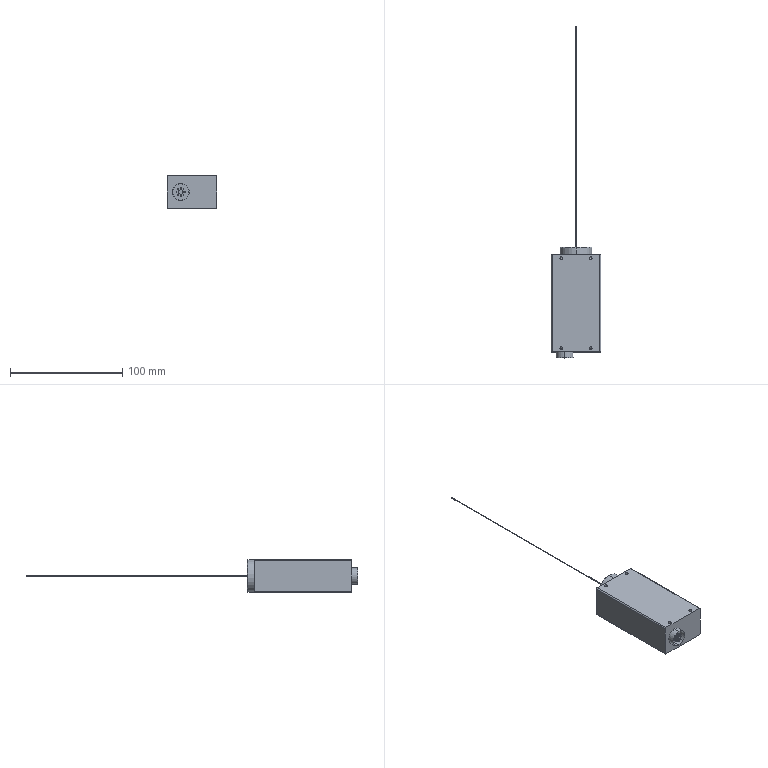Part | STEP file | Camera | 1 solid | 93 faces | box 44 x 295.5 x 29 mm | volume 113476 mm3 | cylinder 54 | plane 27 | cone 8 | torus 4 | commonest cylinder face diameters 0.519 x32 2.5 x8 2 x4 0.5 x2 14.6 x2 15 x2